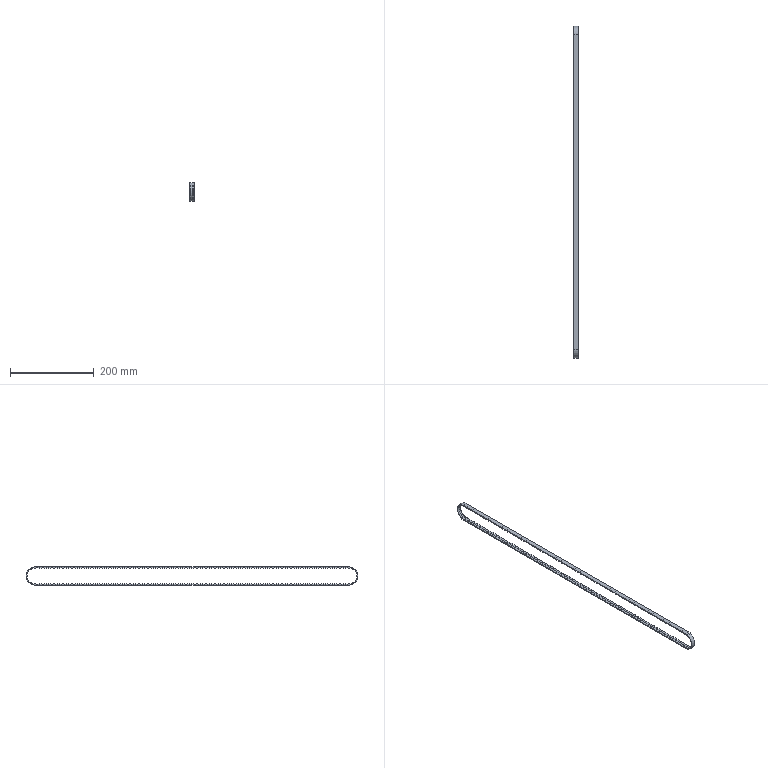Part | NX | features CPROJ 5, DATUM_CSYS 4, EXTRUDE 3, SKETCH 3, EXTRACT_BODY 2, TRIM BODY 2, Container 1, Delete Body 1, Geometry Instance 1, Pattern Geometry 1, UNITE 1 | 1 solid | 614 faces | box 10 x 791 x 43 mm | volume 37818 mm3 | plane 586 | cylinder 28 | commonest cylinder face diameters 37.525 x14 40 x12 43 x2